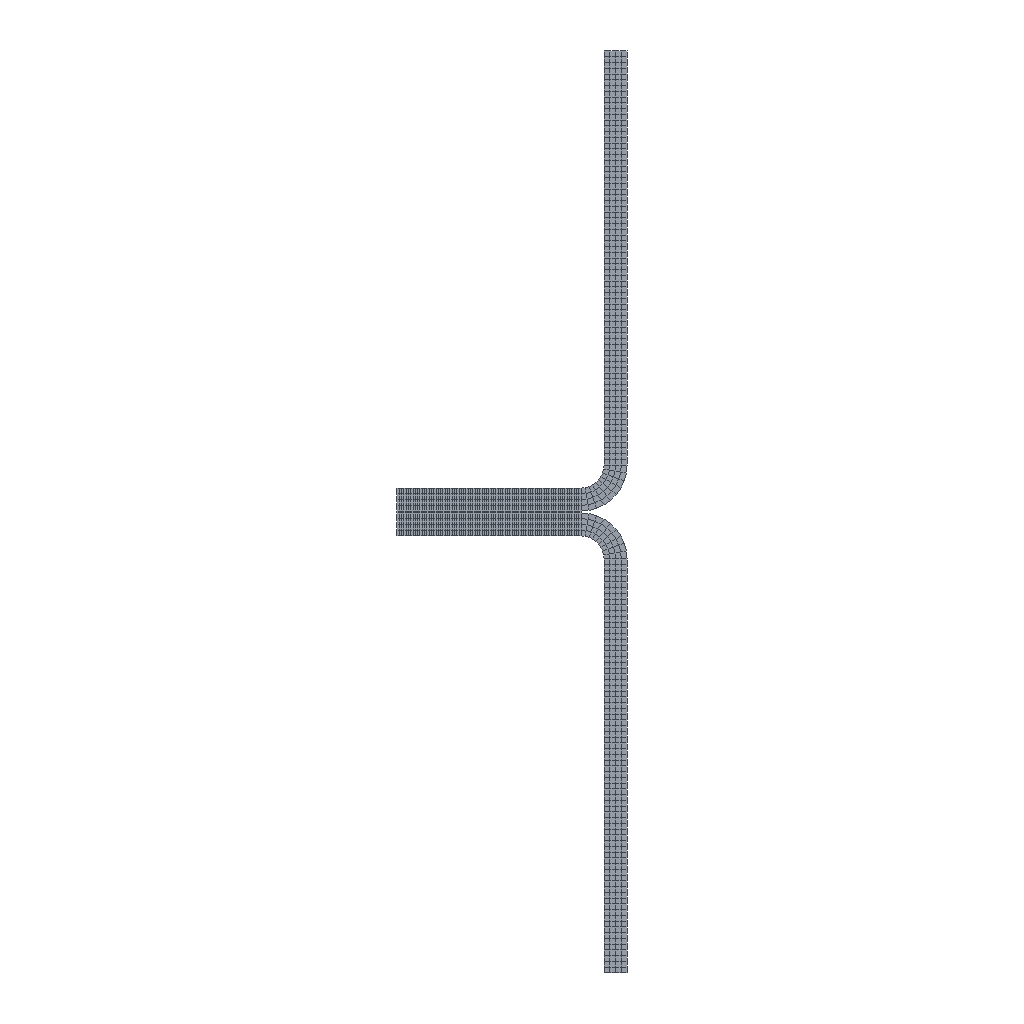Simulation study | abaqus
Set-up summary:
category,name,step,type,value,unit,region
solver,abaqus
solver,version,,,Abaqus/Explicit 3DEXPERIENCE R2017x
units,not stated in the deck,,not stated
analysis,deck,,transient,transient
load_step,Step-1,Step-1,transient
load_step,requested,,,1
mesh,nodes,,,1620
mesh,elements,,,1368
element_type,CPS4R,,plane,1288
element_type,COH2D4,,cohesive,80
load,load commands in deck,,count,1
bc,support commands in deck,,count,3
material,COHESIVE,,in results
material,STEEL,,in results
check,setup vs results,,match,"per instance, exact: element labels, types and connectivity; labels of the nodes the elements use; coordinates not compared"
Abaqus input file, long lists of numbers shortened:
*Heading
** Job name: Job-1 Model name: Model-1
** Generated by: Abaqus/CAE 2017
*Preprint, echo=NO, model=NO, history=NO, contact=NO
**
** PARTS
**
*Part, name=Part-1
*Node
      1,          10.,  -2.08
      2,           9.,  -2.08
** (1618 more lines like these left out)
*Element, type=CPS4R
  1,   1,  17, 673, 164
  2,  17,  18, 674, 673
** (1286 more lines like these left out)
*Element, type=COH2D4
645,   9, 345, 184,   5
646, 345, 346, 185, 184
** (78 more lines like these left out)
*Nset, nset=Set-17, generate
    1,  1620,     1
*Elset, elset=Set-17
    1,    2,    3,    4,    5,    6,    7,    8,    9,   10,   11,   12,   13,   14,   15,   16
   17,   18,   19,   20,   21,   22,   23,   24,   25,   26,   27,   28,   29,   30,   31,   32
** (79 more lines like these left out)
*Nset, nset=Set-18
   5,   7,   9,  10, 184, 185, 186, 187, 188, 189, 190, 191, 192, 193, 194, 195
 196, 197, 198, 199, 200, 201, 202, 203, 204, 205, 206, 207, 208, 209, 210, 211
** (9 more lines like these left out)
*Elset, elset=Set-18, generate
 645,  724,    1
*Nset, nset=Set-28
   5,   7,   9,  10, 184, 185, 186, 187, 188, 189, 190, 191, 192, 193, 194, 195
 196, 197, 198, 199, 200, 201, 202, 203, 204, 205, 206, 207, 208, 209, 210, 211
** (9 more lines like these left out)
*Elset, elset=Set-28, generate
 645,  724,    1
** Section: STEEL
*Solid Section, elset=Set-17, material=STEEL
10.,
** Section: COHESIVE
*Cohesive Section, elset=Set-28, controls=EC-1, material=COHESIVE, response=TRACTION SEPARATION
, 10.
*End Part
**
**
** ASSEMBLY
**
*Assembly, name=Assembly
**
*Instance, name=Part-1-1, part=Part-1
*End Instance
**
*Nset, nset=Set-1, instance=Part-1-1
  3,  4, 91, 92, 93
*Elset, elset=Set-1, instance=Part-1-1, generate
 285,  288,    1
*Nset, nset=Set-2, instance=Part-1-1
  15,  16, 599, 600, 601
*Elset, elset=Set-2, instance=Part-1-1, generate
 1365,  1368,     1
*Nset, nset=Set-3, instance=Part-1-1
  15,  16, 599, 600, 601
*Elset, elset=Set-3, instance=Part-1-1, generate
 1365,  1368,     1
*Nset, nset=_PickedSet7, internal, instance=Part-1-1
    1,    2,    5,    6,    7,    8,    9,   10,   11,   12,   13,   14,   17,   18,   19,  165
  166,  167,  168,  169,  170,  171,  172,  173,  174,  175,  176,  177,  178,  179,  180,  181
** (55 more lines like these left out)
*Elset, elset=_PickedSet7, internal, instance=Part-1-1
  289,  290,  291,  292,  293,  294,  295,  296,  297,  298,  299,  300,  301,  302,  303,  304
  305,  306,  307,  308,  309,  310,  311,  312,  313,  314,  315,  316,  317,  318,  319,  320
** (43 more lines like these left out)
*End Assembly
**
** ELEMENT CONTROLS
**
*Section Controls, name=EC-1, ELEMENT DELETION=YES
1., 1., 1., 0.0001, 1.
*Amplitude, name=Amp-1, smooth=0.05
             0.,              0.,           0.001,              1.,           0.002,              0.,           0.003,              1.
          0.004,              0.,           0.005,              1.,           0.006,              0.,           0.007,              1.
          0.008,              0.,           0.009,              1.,            0.01,              0.,           0.011,              1.
          0.012,              0.,           0.013,              1.,           0.014,              0.,           0.015,              1.
          0.016,              0.,           0.017,              1.,           0.018,              0.,           0.019,              1.
           0.02,              0.,           0.021,              1.,           0.022,              0.,           0.023,              1.
          0.024,              0.,           0.025,              1.,           0.026,              0.,           0.027,              1.
          0.028,              0.,           0.029,              1.,            0.03,              0.,           0.031,              1.
          0.032,              0.,           0.033,              1.,           0.034,              0.,           0.035,              1.
          0.036,              0.,           0.037,              1.,           0.038,              0.,           0.039,              1.
           0.04,              0.,           0.041,              1.,           0.042,              0.,           0.043,              1.
          0.044,              0.,           0.045,              1.,           0.046,              0.,           0.047,              1.
          0.048,              0.,           0.049,              1.,            0.05,              0.,           0.051,              1.
          0.052,              0.,           0.053,              1.,           0.054,              0.,           0.055,              1.
          0.056,              0.,           0.057,              1.,           0.058,              0.,           0.059,              1.
           0.06,              0.,           0.061,              1.,           0.062,              0.,           0.063,              1.
          0.064,              0.,           0.065,              1.,           0.066,              0.,           0.067,              1.
          0.068,              0.,           0.069,              1.,            0.07,              0.,           0.071,              1.
          0.072,              0.,           0.073,              1.,           0.074,              0.,           0.075,              1.
          0.076,              0.,           0.077,              1.,           0.078,              0.,           0.079,              1.
           0.08,              0.,           0.081,              1.,           0.082,              0.,           0.083,              1.
          0.084,              0.,           0.085,              1.,           0.086,              0.,           0.087,              1.
          0.088,              0.,           0.089,              1.,            0.09,              0.,           0.091,              1.
          0.092,              0.,           0.093,              1.,           0.094,              0.,           0.095,              1.
          0.096,              0.,           0.097,              1.,           0.098,              0.,           0.099,              1.
            0.1,              0.,           0.101,              1.,           0.102,              0.,           0.103,              1.
          0.104,              0.,           0.105,              1.,           0.106,              0.,           0.107,              1.
          0.108,              0.,           0.109,              1.,            0.11,              0.,           0.111,              1.
          0.112,              0.,           0.113,              1.,           0.114,              0.,           0.115,              1.
          0.116,              0.,           0.117,              1.,           0.118,              0.,           0.119,              1.
           0.12,              0.,           0.121,              1.,           0.122,              0.,           0.123,              1.
          0.124,              0.,           0.125,              1.,           0.126,              0.,           0.127,              1.
          0.128,              0.,           0.129,              1.,            0.13,              0.,           0.131,              1.
          0.132,              0.,           0.133,              1.,           0.134,              0.,           0.135,              1.
          0.136,              0.,           0.137,              1.,           0.138,              0.,           0.139,              1.
           0.14,              0.,           0.141,              1.,           0.142,              0.,           0.143,              1.
          0.144,              0.,           0.145,              1.,           0.146,              0.,           0.147,              1.
          0.148,              0.,           0.149,              1.,            0.15,              0.,           0.151,              1.
          0.152,              0.,           0.153,              1.,           0.154,              0.,           0.155,              1.
          0.156,              0.,           0.157,              1.,           0.158,              0.,           0.159,              1.
** (211 more lines like these left out)
**
** MATERIALS
**
*Material, name=COHESIVE
*Density
 7.85e-09,
*Depvar
      8,
*User Material, constants=10
 2.5625e+06, 2.5625e+06,        30.,        30.,      10.45,      10.45,         2.,         1.
         5.,        0.1
*Material, name=STEEL
*Density
 7.85e-09,
*Elastic
206000., 0.3
**
** BOUNDARY CONDITIONS
**
** Name: BC-1 Type: 对称/反对称/完全固定
*Boundary
Set-1, ENCASTRE
** Name: BC-2 Type: 位移/转角
*Boundary
Set-2, 1, 1
** ----------------------------------------------------------------
**
** STEP: Step-1
**
*Step, name=Step-1, nlgeom=YES
*Dynamic, Explicit, direct user control
1e-08, 0.04
*Bulk Viscosity
0.06, 1.2
**
** BOUNDARY CONDITIONS
**
** Name: BC-3 Type: 位移/转角
*Boundary, amplitude=Amp-1
Set-3, 2, 2, 0.002
*Adaptive Mesh Controls, name=Ada-1
1., 0., 0.
**
** OUTPUT REQUESTS
**
*Restart, write, number interval=1, time marks=NO
**
** FIELD OUTPUT: F-Output-1
**
*Output, field, time interval=0.0002
*Node Output
RF, RT, U, V
*Element Output, directions=YES
E, MISES, NFORC, PE, PEEQ, PEEQMAX, PEEQT, PEMAG, PEVAVG, S, SDV, SF, STATUS, VE, VEEQ
*Contact Output
CSTRESS,
**
** HISTORY OUTPUT: H-Output-1
**
*Output, history, variable=PRESELECT
*End Step
Results summary:
result,step,Step-1,completed,increments=4000001 time=0.04/0.04
result,analysis,,,transient
result,last_loadstep,,,1
result,primary field,,,U
result,reaction total,,FX,0.1129,model units
result,reaction total,,FY,0.1226,model units
result,reaction total,,FZ,0.0,model units